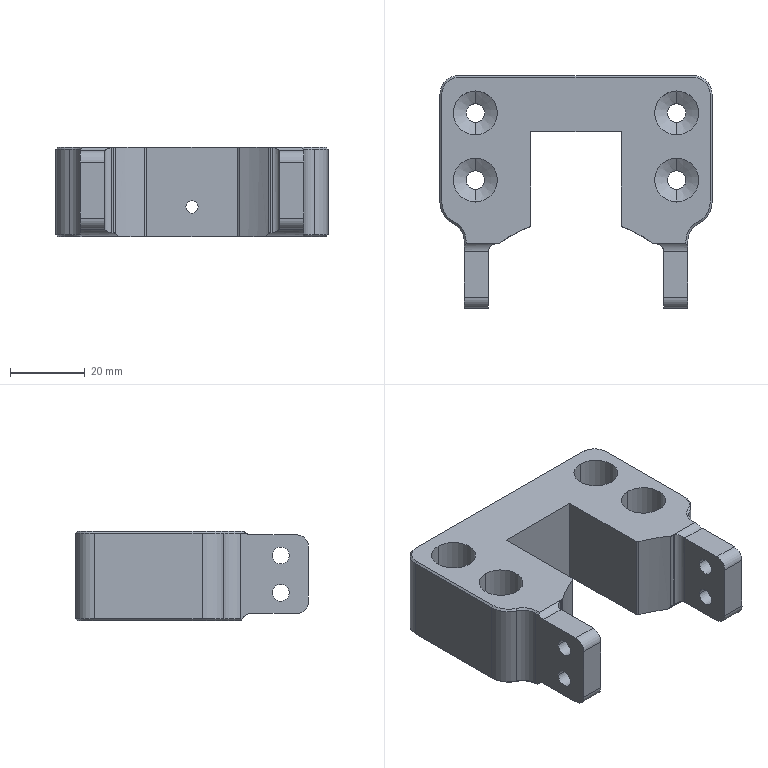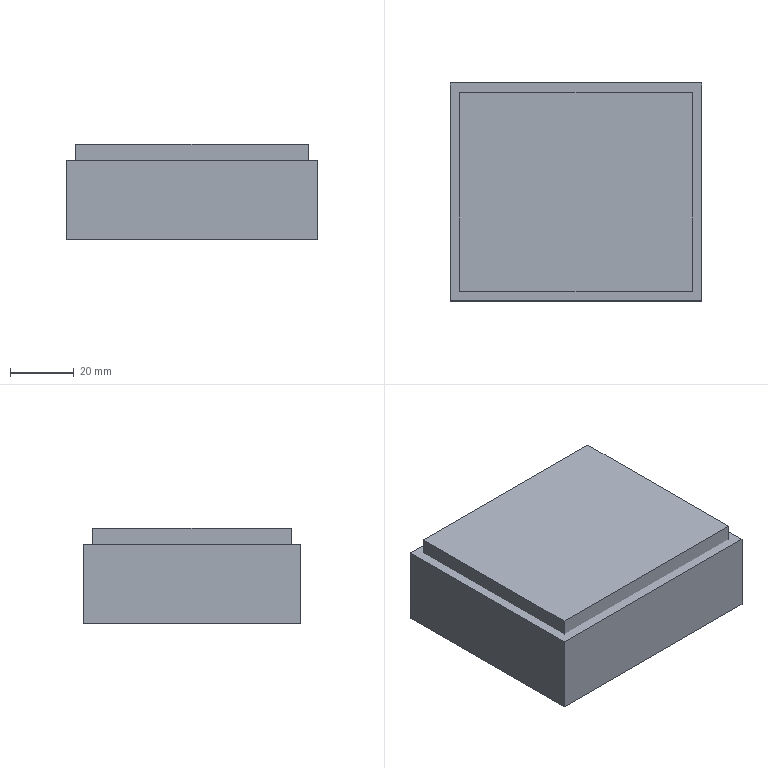CAM job | NX | 3-axis milling, drilling | part box 73 x 62.4 x 24 mm | stock box 79 x 68.4 x 30 mm
Tools:
number,name,description,diameter,corner_radius,flute_length,length,flutes
1,D63,Milling Tool-5 Parameters,63.0,0.0,50.0,75.0,2
7,D6A45,Milling Tool-5 Parameters,6.0,0.0,3.0,3.0,2
15,5.0ZT,Drilling Tool,5.0,0.0,35.0,50.0,2
12,11.8ZT,Drilling Tool,11.8,0.0,35.0,50.0,2
10,D10,Milling Tool-5 Parameters,10.0,0.0,50.0,75.0,2
11,D10JING,Milling Tool-5 Parameters,10.0,0.0,50.0,75.0,2
4,D4,Milling Tool-5 Parameters,4.0,0.0,50.0,75.0,2
5,D6R0.5,Milling Tool-5 Parameters,6.0,0.5,50.0,75.0,2
Operations:
program,operation,operation_type,tool,method,geometry_group,spindle_rpm,surface_speed,feed_per_tooth,feed_cut,feed_plunge,cut_length_mm,path_length_mm,cut_time_min,machine_time_min
1-75-65-30-BLANK-G54G55,FLOOR_WALL,VolumeBased25DMillingOperation,D63,METHOD,A,6500.0,1286.0,0.0962,1250.0,100.0,339.197,393.197,0.2714,0.2768
1-75-65-30-BLANK-G54G55,FLOOR_WALL_COPY_1,VolumeBased25DMillingOperation,D63,METHOD,AA,6500.0,1286.0,0.0962,1250.0,100.0,339.197,393.197,0.2714,0.2768
1-75-65-30-BLANK-G54G55,DRILLING_COPY_1,Operation,D6A45,METHOD,A,3000.0,56.0,0.0333,200.0,0.0,16.0,191.58,0.08,0.0976
1-75-65-30-BLANK-G54G55,DRILLING_COPY_1_COPY_1,Operation,D6A45,METHOD,AA,3000.0,56.0,0.0333,200.0,0.0,16.0,191.58,0.08,0.0976
1-75-65-30-BLANK-G54G55,DRILLING_COPY_1_COPY,Operation,5.0ZT,METHOD,A,2000.0,36.0,0.05,200.0,0.0,120.009,399.597,0.6,0.628
1-75-65-30-BLANK-G54G55,DRILLING_COPY_1_COPY_COPY_1,Operation,5.0ZT,METHOD,AA,2000.0,36.0,0.05,200.0,0.0,120.009,399.597,0.6,0.628
1-75-65-30-BLANK-G54G55,DRILLING_COPY_1_COPY_COPY,Operation,11.8ZT,METHOD,A,1500.0,55.0,0.0667,200.0,0.0,86.18,331.94,0.4309,0.4555
1-75-65-30-BLANK-G54G55,DRILLING_COPY_1_COPY_COPY_COPY,Operation,11.8ZT,METHOD,AA,1500.0,55.0,0.0667,200.0,0.0,86.18,331.94,0.4309,0.4555
1-75-65-30-BLANK-G54G55,ADAPTIVE_MILLING,CavityMilling,D10,METHOD,A,8000.0,251.0,0.2188,3500.0,1000.0,10082.562,10348.724,2.885,2.912
1-75-65-30-BLANK-G54G55,ADAPTIVE_MILLING_COPY,CavityMilling,D10,METHOD,AA,8000.0,251.0,0.2188,3500.0,1000.0,10082.562,10348.724,2.885,2.912
1-75-65-30-BLANK-G54G55,ZLEVEL_PROFILE_COPY_COPY_1,ZLevelMilling,D10JING,METHOD,A,8000.0,251.0,0.05,800.0,100.0,752.149,858.618,0.9402,0.9508
1-75-65-30-BLANK-G54G55,FLOOR_WALL_1_1_COPY,VolumeBased25DMillingOperation,D10JING,METHOD,A,7000.0,219.0,0.0893,1250.0,100.0,170.109,342.483,0.1361,0.1533
1-75-65-30-BLANK-G54G55,ZLEVEL_PROFILE_COPY_COPY_1_COPY,ZLevelMilling,D10JING,METHOD,AA,8000.0,251.0,0.05,800.0,100.0,752.149,858.618,0.9402,0.9508
1-75-65-30-BLANK-G54G55,FLOOR_WALL_1_1_COPY_COPY_1,VolumeBased25DMillingOperation,D10JING,METHOD,AA,7000.0,219.0,0.0893,1250.0,100.0,170.109,342.483,0.1361,0.1533
1-75-65-30-BLANK-G54G55,ZLEVEL_PROFILE_COPY_1_COPY_1_COPY_1_1_COPY_COPY_COPY_1,ZLevelMilling,D4,METHOD,A,7000.0,87.0,0.1071,1500.0,800.0,2069.041,3590.61,1.556,1.708
1-75-65-30-BLANK-G54G55,ZLEVEL_PROFILE_COPY_1_COPY_1_COPY_1_1_COPY_COPY_COPY_1_COPY,ZLevelMilling,D4,METHOD,AA,7000.0,87.0,0.1071,1500.0,800.0,2069.041,3590.61,1.556,1.708
1-75-65-30-BLANK-G54G55,ZLEVEL_PROFILE_COPY_1_COPY_1_COPY_1_1_COPY_1,ZLevelMilling,D6R0.5,METHOD,A,8000.0,150.0,0.1875,3000.0,800.0,425.502,591.89,0.1474,0.1641
1-75-65-30-BLANK-G54G55,ZLEVEL_PROFILE_COPY_1_COPY_1_COPY_1_1_COPY_1_COPY,ZLevelMilling,D6R0.5,METHOD,A,8000.0,150.0,0.1875,3000.0,800.0,849.882,1019.166,0.2888,0.3058
1-75-65-30-BLANK-G54G55,ZLEVEL_PROFILE_COPY_1_COPY_1_COPY_1_1_COPY_1_COPY_2,ZLevelMilling,D6R0.5,METHOD,AA,8000.0,150.0,0.1875,3000.0,800.0,425.502,591.89,0.1474,0.1641
1-75-65-30-BLANK-G54G55,ZLEVEL_PROFILE_COPY_1_COPY_1_COPY_1_1_COPY_1_COPY_COPY_1,ZLevelMilling,D6R0.5,METHOD,AA,8000.0,150.0,0.1875,3000.0,800.0,849.882,1019.166,0.2888,0.3058
1-75-65-30-BLANK-G54G55,ZLEVEL_PROFILE_1_COPY_1_COPY_COPY_1_COPY,ZLevelMilling,D6A45,METHOD,A,7500.0,141.0,0.0667,1000.0,100.0,451.616,1069.429,0.4516,0.5134
1-75-65-30-BLANK-G54G55,ZLEVEL_PROFILE_1_COPY_1_COPY_COPY_1_COPY_COPY_1,ZLevelMilling,D6A45,METHOD,AA,7500.0,141.0,0.0667,1000.0,100.0,451.616,1069.429,0.4516,0.5134
2-75-65-30-BLANK-G54G55,FLOOR_WALL_COPY,VolumeBased25DMillingOperation,D63,METHOD,B,6500.0,1286.0,0.0962,1250.0,100.0,1927.182,2407.168,1.542,1.59
2-75-65-30-BLANK-G54G55,FLOOR_WALL_COPY_COPY,VolumeBased25DMillingOperation,D63,METHOD,BB,6500.0,1286.0,0.0962,1250.0,100.0,1927.182,2407.168,1.542,1.59
2-75-65-30-BLANK-G54G55,FLOOR_WALL_1_1_COPY_COPY,VolumeBased25DMillingOperation,D10JING,METHOD,B,7000.0,219.0,0.0893,1250.0,100.0,340.217,657.644,0.2722,0.3039
2-75-65-30-BLANK-G54G55,FLOOR_WALL_1_1_COPY_COPY_COPY,VolumeBased25DMillingOperation,D10JING,METHOD,BB,7000.0,219.0,0.0893,1250.0,100.0,340.217,657.644,0.2722,0.3039
2-75-65-30-BLANK-G54G55,ZLEVEL_PROFILE_COPY_1_COPY_1_COPY_1_1_COPY_1_COPY_1,ZLevelMilling,D6R0.5,METHOD,B,8000.0,150.0,0.1875,3000.0,800.0,693.919,924.729,0.2399,0.263
2-75-65-30-BLANK-G54G55,ZLEVEL_PROFILE_COPY_1_COPY_1_COPY_1_1_COPY_1_COPY_COPY,ZLevelMilling,D6R0.5,METHOD,B,8000.0,150.0,0.1875,3000.0,800.0,850.908,1043.006,0.2892,0.3084
2-75-65-30-BLANK-G54G55,ZLEVEL_PROFILE_COPY_1_COPY_1_COPY_1_1_COPY_1_COPY_1_COPY,ZLevelMilling,D6R0.5,METHOD,BB,8000.0,150.0,0.1875,3000.0,800.0,693.919,924.729,0.2399,0.263
2-75-65-30-BLANK-G54G55,ZLEVEL_PROFILE_COPY_1_COPY_1_COPY_1_1_COPY_1_COPY_COPY_COPY,ZLevelMilling,D6R0.5,METHOD,BB,8000.0,150.0,0.1875,3000.0,800.0,850.908,1043.006,0.2892,0.3084
2-75-65-30-BLANK-G54G55,ZLEVEL_PROFILE_1_COPY_1_COPY_COPY_1_COPY_COPY,ZLevelMilling,D6A45,METHOD,B,7500.0,141.0,0.0667,1000.0,100.0,296.784,860.142,0.2968,0.3531
2-75-65-30-BLANK-G54G55,ZLEVEL_PROFILE_1_COPY_1_COPY_COPY_1_COPY_COPY_COPY,ZLevelMilling,D6A45,METHOD,B,7500.0,141.0,0.0667,1000.0,100.0,68.734,410.66,0.0687,0.1029
2-75-65-30-BLANK-G54G55,ZLEVEL_PROFILE_1_COPY_1_COPY_COPY_1_COPY_COPY_COPY_1,ZLevelMilling,D6A45,METHOD,BB,7500.0,141.0,0.0667,1000.0,100.0,296.784,860.142,0.2968,0.3531
2-75-65-30-BLANK-G54G55,ZLEVEL_PROFILE_1_COPY_1_COPY_COPY_1_COPY_COPY_COPY_COPY,ZLevelMilling,D6A45,METHOD,BB,7500.0,141.0,0.0667,1000.0,100.0,68.734,410.66,0.0687,0.1029